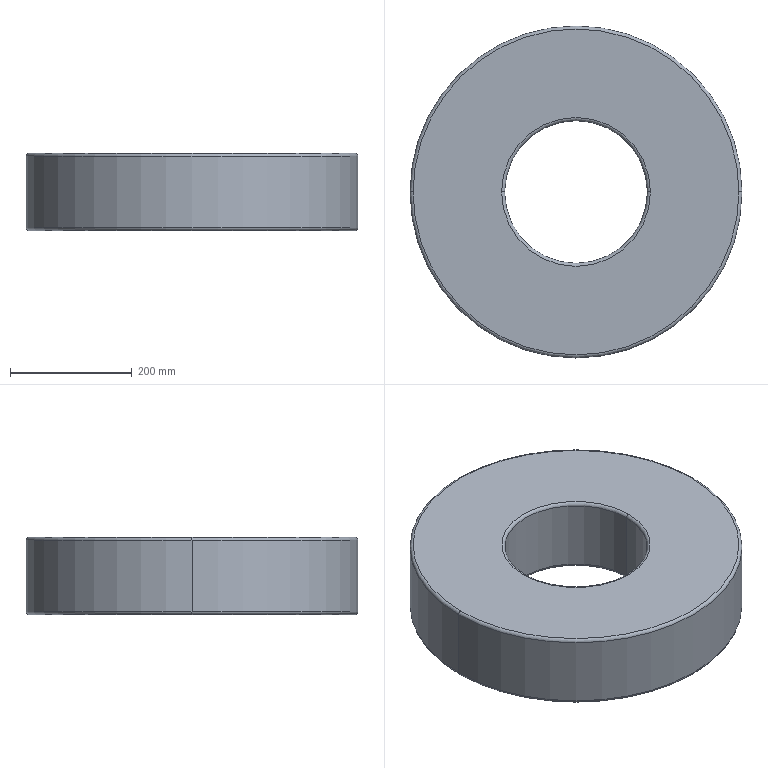Part | SolidWorks | features Extrusion 1, Fillet 1 | 1 solid | 14 faces | box 546.1 x 546.1 x 127 mm | volume 24214209 mm3 | torus 8 | cylinder 4 | plane 2 | commonest cylinder face diameters 234.95 x2 546.1 x2
STEP:
#1=CARTESIAN_POINT('',(-273.05,0.,122.));
#2=VERTEX_POINT('',#1);
#3=CARTESIAN_POINT('',(273.05,0.,122.));
#4=VERTEX_POINT('',#3);
#5=CARTESIAN_POINT('',(0.,0.,122.));
#6=DIRECTION('',(0.,0.,-1.));
#7=DIRECTION('',(1.,0.,0.));
#8=AXIS2_PLACEMENT_3D('',#5,#6,#7);
#9=CIRCLE('',#8,273.05);
#10=EDGE_CURVE('',#2,#4,#9,.T.);
#11=ORIENTED_EDGE('',*,*,#10,.F.);
#12=CARTESIAN_POINT('',(-268.05,0.,127.));
#13=VERTEX_POINT('',#12);
#14=CARTESIAN_POINT('',(-268.05,0.,122.));
#15=DIRECTION('',(0.,1.,0.));
#16=DIRECTION('',(-1.,0.,0.));
#17=AXIS2_PLACEMENT_3D('',#14,#15,#16);
#18=CIRCLE('',#17,5.);
#19=EDGE_CURVE('',#2,#13,#18,.T.);
#20=ORIENTED_EDGE('',*,*,#19,.T.);
#21=CARTESIAN_POINT('',(268.05,0.,127.));
#22=VERTEX_POINT('',#21);
#23=CARTESIAN_POINT('',(0.,0.,127.));
#24=DIRECTION('',(0.,0.,1.));
#25=DIRECTION('',(1.,0.,0.));
#26=AXIS2_PLACEMENT_3D('',#23,#24,#25);
#27=CIRCLE('',#26,268.05);
#28=EDGE_CURVE('',#22,#13,#27,.T.);
#29=ORIENTED_EDGE('',*,*,#28,.F.);
#30=CARTESIAN_POINT('',(268.05,0.,122.));
#31=DIRECTION('',(0.,-1.,0.));
#32=DIRECTION('',(0.,0.,-1.));
#33=AXIS2_PLACEMENT_3D('',#30,#31,#32);
#34=CIRCLE('',#33,5.);
#35=EDGE_CURVE('',#4,#22,#34,.T.);
#36=ORIENTED_EDGE('',*,*,#35,.F.);
#37=EDGE_LOOP('',(#11,#20,#29,#36));
#38=FACE_OUTER_BOUND('',#37,.T.);
#39=CARTESIAN_POINT('',(0.,0.,122.));
#40=DIRECTION('',(0.,0.,1.));
#41=DIRECTION('',(1.,0.,0.));
#42=AXIS2_PLACEMENT_3D('',#39,#40,#41);
#43=TOROIDAL_SURFACE('',#42,268.05,5.);
#44=ADVANCED_FACE('',(#38),#43,.T.);
#45=CARTESIAN_POINT('',(-122.475,0.,127.));
#46=VERTEX_POINT('',#45);
#47=CARTESIAN_POINT('',(122.475,0.,127.));
#48=VERTEX_POINT('',#47);
#49=CARTESIAN_POINT('',(0.,0.,127.));
#50=DIRECTION('',(0.,0.,-1.));
#51=DIRECTION('',(1.,0.,0.));
#52=AXIS2_PLACEMENT_3D('',#49,#50,#51);
#53=CIRCLE('',#52,122.475);
#54=EDGE_CURVE('',#46,#48,#53,.T.);
#55=ORIENTED_EDGE('',*,*,#54,.F.);
#56=CARTESIAN_POINT('',(-117.475,0.,122.));
#57=VERTEX_POINT('',#56);
#58=CARTESIAN_POINT('',(-122.475,0.,122.));
#59=DIRECTION('',(0.,1.,0.));
#60=DIRECTION('',(-1.,0.,0.));
#61=AXIS2_PLACEMENT_3D('',#58,#59,#60);
#62=CIRCLE('',#61,5.);
#63=EDGE_CURVE('',#46,#57,#62,.T.);
#64=ORIENTED_EDGE('',*,*,#63,.T.);
#65=CARTESIAN_POINT('',(117.475,0.,122.));
#66=VERTEX_POINT('',#65);
#67=CARTESIAN_POINT('',(0.,0.,122.));
#68=DIRECTION('',(0.,0.,1.));
#69=DIRECTION('',(1.,0.,0.));
#70=AXIS2_PLACEMENT_3D('',#67,#68,#69);
#71=CIRCLE('',#70,117.475);
#72=EDGE_CURVE('',#66,#57,#71,.T.);
#73=ORIENTED_EDGE('',*,*,#72,.F.);
#74=CARTESIAN_POINT('',(122.475,0.,122.));
#75=DIRECTION('',(0.,-1.,0.));
#76=DIRECTION('',(0.,0.,-1.));
#77=AXIS2_PLACEMENT_3D('',#74,#75,#76);
#78=CIRCLE('',#77,5.);
#79=EDGE_CURVE('',#48,#66,#78,.T.);
#80=ORIENTED_EDGE('',*,*,#79,.F.);
#81=EDGE_LOOP('',(#55,#64,#73,#80));
#82=FACE_OUTER_BOUND('',#81,.T.);
#83=CARTESIAN_POINT('',(0.,0.,122.));
#84=DIRECTION('',(0.,0.,1.));
#85=DIRECTION('',(1.,0.,0.));
#86=AXIS2_PLACEMENT_3D('',#83,#84,#85);
#87=TOROIDAL_SURFACE('',#86,122.475,5.);
#88=ADVANCED_FACE('',(#82),#87,.T.);
#89=CARTESIAN_POINT('',(-117.475,0.,5.));
#90=VERTEX_POINT('',#89);
#91=CARTESIAN_POINT('',(117.475,0.,5.));
#92=VERTEX_POINT('',#91);
#93=CARTESIAN_POINT('',(0.,0.,5.));
#94=DIRECTION('',(0.,0.,-1.));
#95=DIRECTION('',(1.,0.,0.));
#96=AXIS2_PLACEMENT_3D('',#93,#94,#95);
#97=CIRCLE('',#96,117.475);
#98=EDGE_CURVE('',#90,#92,#97,.T.);
#99=ORIENTED_EDGE('',*,*,#98,.F.);
#100=CARTESIAN_POINT('',(-122.475,0.,0.));
#101=VERTEX_POINT('',#100);
#102=CARTESIAN_POINT('',(-122.475,0.,5.));
#103=DIRECTION('',(0.,1.,0.));
#104=DIRECTION('',(-1.,0.,0.));
#105=AXIS2_PLACEMENT_3D('',#102,#103,#104);
#106=CIRCLE('',#105,5.);
#107=EDGE_CURVE('',#90,#101,#106,.T.);
#108=ORIENTED_EDGE('',*,*,#107,.T.);
#109=CARTESIAN_POINT('',(122.475,0.,0.));
#110=VERTEX_POINT('',#109);
#111=CARTESIAN_POINT('',(0.,0.,0.));
#112=DIRECTION('',(0.,0.,1.));
#113=DIRECTION('',(1.,0.,0.));
#114=AXIS2_PLACEMENT_3D('',#111,#112,#113);
#115=CIRCLE('',#114,122.475);
#116=EDGE_CURVE('',#110,#101,#115,.T.);
#117=ORIENTED_EDGE('',*,*,#116,.F.);
#118=CARTESIAN_POINT('',(122.475,0.,5.));
#119=DIRECTION('',(0.,-1.,0.));
#120=DIRECTION('',(0.,0.,-1.));
#121=AXIS2_PLACEMENT_3D('',#118,#119,#120);
#122=CIRCLE('',#121,5.);
#123=EDGE_CURVE('',#92,#110,#122,.T.);
#124=ORIENTED_EDGE('',*,*,#123,.F.);
#125=EDGE_LOOP('',(#99,#108,#117,#124));
#126=FACE_OUTER_BOUND('',#125,.T.);
#127=CARTESIAN_POINT('',(0.,0.,5.));
#128=DIRECTION('',(0.,0.,1.));
#129=DIRECTION('',(1.,0.,0.));
#130=AXIS2_PLACEMENT_3D('',#127,#128,#129);
#131=TOROIDAL_SURFACE('',#130,122.475,5.);
#132=ADVANCED_FACE('',(#126),#131,.T.);
#133=CARTESIAN_POINT('',(-268.05,0.,0.));
#134=VERTEX_POINT('',#133);
#135=CARTESIAN_POINT('',(268.05,0.,0.));
#136=VERTEX_POINT('',#135);
#137=CARTESIAN_POINT('',(0.,0.,0.));
#138=DIRECTION('',(0.,0.,-1.));
#139=DIRECTION('',(1.,0.,0.));
#140=AXIS2_PLACEMENT_3D('',#137,#138,#139);
#141=CIRCLE('',#140,268.05);
#142=EDGE_CURVE('',#134,#136,#141,.T.);
#143=ORIENTED_EDGE('',*,*,#142,.F.);
#144=CARTESIAN_POINT('',(-273.05,0.,5.));
#145=VERTEX_POINT('',#144);
#146=CARTESIAN_POINT('',(-268.05,0.,5.));
#147=DIRECTION('',(0.,1.,0.));
#148=DIRECTION('',(-1.,0.,0.));
#149=AXIS2_PLACEMENT_3D('',#146,#147,#148);
#150=CIRCLE('',#149,5.);
#151=EDGE_CURVE('',#134,#145,#150,.T.);
#152=ORIENTED_EDGE('',*,*,#151,.T.);
#153=CARTESIAN_POINT('',(273.05,0.,5.));
#154=VERTEX_POINT('',#153);
#155=CARTESIAN_POINT('',(0.,0.,5.));
#156=DIRECTION('',(0.,0.,1.));
#157=DIRECTION('',(1.,0.,0.));
#158=AXIS2_PLACEMENT_3D('',#155,#156,#157);
#159=CIRCLE('',#158,273.05);
#160=EDGE_CURVE('',#154,#145,#159,.T.);
#161=ORIENTED_EDGE('',*,*,#160,.F.);
#162=CARTESIAN_POINT('',(268.05,0.,5.));
#163=DIRECTION('',(0.,-1.,0.));
#164=DIRECTION('',(0.,0.,-1.));
#165=AXIS2_PLACEMENT_3D('',#162,#163,#164);
#166=CIRCLE('',#165,5.);
#167=EDGE_CURVE('',#136,#154,#166,.T.);
#168=ORIENTED_EDGE('',*,*,#167,.F.);
#169=EDGE_LOOP('',(#143,#152,#161,#168));
#170=FACE_OUTER_BOUND('',#169,.T.);
#171=CARTESIAN_POINT('',(0.,0.,5.));
#172=DIRECTION('',(0.,0.,1.));
#173=DIRECTION('',(1.,0.,0.));
#174=AXIS2_PLACEMENT_3D('',#171,#172,#173);
#175=TOROIDAL_SURFACE('',#174,268.05,5.);
#176=ADVANCED_FACE('',(#170),#175,.T.);
#177=CARTESIAN_POINT('',(0.,0.,122.));
#178=DIRECTION('',(0.,0.,1.));
#179=DIRECTION('',(1.,0.,0.));
#180=AXIS2_PLACEMENT_3D('',#177,#178,#179);
#181=CIRCLE('',#180,117.475);
#182=EDGE_CURVE('',#57,#66,#181,.T.);
#183=ORIENTED_EDGE('',*,*,#182,.T.);
#184=CARTESIAN_POINT('',(117.475,0.,127.));
#185=DIRECTION('',(0.,0.,-1.));
#186=VECTOR('',#185,1000.);
#187=LINE('',#184,#186);
#188=EDGE_CURVE('',#66,#92,#187,.T.);
#189=ORIENTED_EDGE('',*,*,#188,.T.);
#190=CARTESIAN_POINT('',(0.,0.,5.));
#191=DIRECTION('',(0.,0.,-1.));
#192=DIRECTION('',(1.,0.,0.));
#193=AXIS2_PLACEMENT_3D('',#190,#191,#192);
#194=CIRCLE('',#193,117.475);
#195=EDGE_CURVE('',#92,#90,#194,.T.);
#196=ORIENTED_EDGE('',*,*,#195,.T.);
#197=CARTESIAN_POINT('',(-117.475,0.,127.));
#198=DIRECTION('',(0.,0.,-1.));
#199=VECTOR('',#198,1000.);
#200=LINE('',#197,#199);
#201=EDGE_CURVE('',#57,#90,#200,.T.);
#202=ORIENTED_EDGE('',*,*,#201,.F.);
#203=EDGE_LOOP('',(#183,#189,#196,#202));
#204=FACE_OUTER_BOUND('',#203,.T.);
#205=CARTESIAN_POINT('',(0.,0.,127.));
#206=DIRECTION('',(0.,0.,-1.));
#207=DIRECTION('',(-1.,0.,0.));
#208=AXIS2_PLACEMENT_3D('',#205,#206,#207);
#209=CYLINDRICAL_SURFACE('',#208,117.475);
#210=ADVANCED_FACE('',(#204),#209,.F.);
#211=ORIENTED_EDGE('',*,*,#10,.T.);
#212=CARTESIAN_POINT('',(273.05,0.,127.));
#213=DIRECTION('',(0.,0.,-1.));
#214=VECTOR('',#213,1000.);
#215=LINE('',#212,#214);
#216=EDGE_CURVE('',#4,#154,#215,.T.);
#217=ORIENTED_EDGE('',*,*,#216,.T.);
#218=ORIENTED_EDGE('',*,*,#160,.T.);
#219=CARTESIAN_POINT('',(-273.05,0.,127.));
#220=DIRECTION('',(0.,0.,-1.));
#221=VECTOR('',#220,1000.);
#222=LINE('',#219,#221);
#223=EDGE_CURVE('',#2,#145,#222,.T.);
#224=ORIENTED_EDGE('',*,*,#223,.F.);
#225=EDGE_LOOP('',(#211,#217,#218,#224));
#226=FACE_OUTER_BOUND('',#225,.T.);
#227=CARTESIAN_POINT('',(0.,0.,127.));
#228=DIRECTION('',(0.,0.,-1.));
#229=DIRECTION('',(-1.,0.,0.));
#230=AXIS2_PLACEMENT_3D('',#227,#228,#229);
#231=CYLINDRICAL_SURFACE('',#230,273.05);
#232=ADVANCED_FACE('',(#226),#231,.T.);
#233=CARTESIAN_POINT('',(0.,0.,127.));
#234=DIRECTION('',(0.,0.,-1.));
#235=DIRECTION('',(1.,0.,0.));
#236=AXIS2_PLACEMENT_3D('',#233,#234,#235);
#237=CIRCLE('',#236,122.475);
#238=EDGE_CURVE('',#48,#46,#237,.T.);
#239=ORIENTED_EDGE('',*,*,#238,.T.);
#240=ORIENTED_EDGE('',*,*,#54,.T.);
#241=EDGE_LOOP('',(#239,#240));
#242=FACE_BOUND('',#241,.T.);
#243=ORIENTED_EDGE('',*,*,#28,.T.);
#244=CARTESIAN_POINT('',(0.,0.,127.));
#245=DIRECTION('',(0.,0.,1.));
#246=DIRECTION('',(1.,0.,0.));
#247=AXIS2_PLACEMENT_3D('',#244,#245,#246);
#248=CIRCLE('',#247,268.05);
#249=EDGE_CURVE('',#13,#22,#248,.T.);
#250=ORIENTED_EDGE('',*,*,#249,.T.);
#251=EDGE_LOOP('',(#243,#250));
#252=FACE_OUTER_BOUND('',#251,.T.);
#253=CARTESIAN_POINT('',(0.,0.,127.));
#254=DIRECTION('',(0.,0.,1.));
#255=DIRECTION('',(1.,0.,0.));
#256=AXIS2_PLACEMENT_3D('',#253,#254,#255);
#257=PLANE('',#256);
#258=ADVANCED_FACE('',(#242,#252),#257,.T.);
#259=CARTESIAN_POINT('',(0.,0.,0.));
#260=DIRECTION('',(0.,0.,-1.));
#261=DIRECTION('',(1.,0.,0.));
#262=AXIS2_PLACEMENT_3D('',#259,#260,#261);
#263=CIRCLE('',#262,268.05);
#264=EDGE_CURVE('',#136,#134,#263,.T.);
#265=ORIENTED_EDGE('',*,*,#264,.T.);
#266=ORIENTED_EDGE('',*,*,#142,.T.);
#267=EDGE_LOOP('',(#265,#266));
#268=FACE_OUTER_BOUND('',#267,.T.);
#269=ORIENTED_EDGE('',*,*,#116,.T.);
#270=CARTESIAN_POINT('',(0.,0.,0.));
#271=DIRECTION('',(0.,0.,1.));
#272=DIRECTION('',(1.,0.,0.));
#273=AXIS2_PLACEMENT_3D('',#270,#271,#272);
#274=CIRCLE('',#273,122.475);
#275=EDGE_CURVE('',#101,#110,#274,.T.);
#276=ORIENTED_EDGE('',*,*,#275,.T.);
#277=EDGE_LOOP('',(#269,#276));
#278=FACE_BOUND('',#277,.T.);
#279=CARTESIAN_POINT('',(0.,0.,0.));
#280=DIRECTION('',(0.,0.,1.));
#281=DIRECTION('',(1.,0.,0.));
#282=AXIS2_PLACEMENT_3D('',#279,#280,#281);
#283=PLANE('',#282);
#284=ADVANCED_FACE('',(#268,#278),#283,.F.);
#285=ORIENTED_EDGE('',*,*,#216,.F.);
#286=CARTESIAN_POINT('',(0.,0.,122.));
#287=DIRECTION('',(0.,0.,-1.));
#288=DIRECTION('',(1.,0.,0.));
#289=AXIS2_PLACEMENT_3D('',#286,#287,#288);
#290=CIRCLE('',#289,273.05);
#291=EDGE_CURVE('',#4,#2,#290,.T.);
#292=ORIENTED_EDGE('',*,*,#291,.T.);
#293=ORIENTED_EDGE('',*,*,#223,.T.);
#294=CARTESIAN_POINT('',(0.,0.,5.));
#295=DIRECTION('',(0.,0.,1.));
#296=DIRECTION('',(1.,0.,0.));
#297=AXIS2_PLACEMENT_3D('',#294,#295,#296);
#298=CIRCLE('',#297,273.05);
#299=EDGE_CURVE('',#145,#154,#298,.T.);
#300=ORIENTED_EDGE('',*,*,#299,.T.);
#301=EDGE_LOOP('',(#285,#292,#293,#300));
#302=FACE_OUTER_BOUND('',#301,.T.);
#303=CARTESIAN_POINT('',(0.,0.,127.));
#304=DIRECTION('',(0.,0.,-1.));
#305=DIRECTION('',(-1.,0.,0.));
#306=AXIS2_PLACEMENT_3D('',#303,#304,#305);
#307=CYLINDRICAL_SURFACE('',#306,273.05);
#308=ADVANCED_FACE('',(#302),#307,.T.);
#309=ORIENTED_EDGE('',*,*,#188,.F.);
#310=ORIENTED_EDGE('',*,*,#72,.T.);
#311=ORIENTED_EDGE('',*,*,#201,.T.);
#312=ORIENTED_EDGE('',*,*,#98,.T.);
#313=EDGE_LOOP('',(#309,#310,#311,#312));
#314=FACE_OUTER_BOUND('',#313,.T.);
#315=CARTESIAN_POINT('',(0.,0.,127.));
#316=DIRECTION('',(0.,0.,-1.));
#317=DIRECTION('',(-1.,0.,0.));
#318=AXIS2_PLACEMENT_3D('',#315,#316,#317);
#319=CYLINDRICAL_SURFACE('',#318,117.475);
#320=ADVANCED_FACE('',(#314),#319,.F.);
#321=ORIENTED_EDGE('',*,*,#151,.F.);
#322=ORIENTED_EDGE('',*,*,#264,.F.);
#323=ORIENTED_EDGE('',*,*,#167,.T.);
#324=ORIENTED_EDGE('',*,*,#299,.F.);
#325=EDGE_LOOP('',(#321,#322,#323,#324));
#326=FACE_OUTER_BOUND('',#325,.T.);
#327=CARTESIAN_POINT('',(0.,0.,5.));
#328=DIRECTION('',(0.,0.,1.));
#329=DIRECTION('',(1.,0.,0.));
#330=AXIS2_PLACEMENT_3D('',#327,#328,#329);
#331=TOROIDAL_SURFACE('',#330,268.05,5.);
#332=ADVANCED_FACE('',(#326),#331,.T.);
#333=ORIENTED_EDGE('',*,*,#107,.F.);
#334=ORIENTED_EDGE('',*,*,#195,.F.);
#335=ORIENTED_EDGE('',*,*,#123,.T.);
#336=ORIENTED_EDGE('',*,*,#275,.F.);
#337=EDGE_LOOP('',(#333,#334,#335,#336));
#338=FACE_OUTER_BOUND('',#337,.T.);
#339=CARTESIAN_POINT('',(0.,0.,5.));
#340=DIRECTION('',(0.,0.,1.));
#341=DIRECTION('',(1.,0.,0.));
#342=AXIS2_PLACEMENT_3D('',#339,#340,#341);
#343=TOROIDAL_SURFACE('',#342,122.475,5.);
#344=ADVANCED_FACE('',(#338),#343,.T.);
#345=ORIENTED_EDGE('',*,*,#63,.F.);
#346=ORIENTED_EDGE('',*,*,#238,.F.);
#347=ORIENTED_EDGE('',*,*,#79,.T.);
#348=ORIENTED_EDGE('',*,*,#182,.F.);
#349=EDGE_LOOP('',(#345,#346,#347,#348));
#350=FACE_OUTER_BOUND('',#349,.T.);
#351=CARTESIAN_POINT('',(0.,0.,122.));
#352=DIRECTION('',(0.,0.,1.));
#353=DIRECTION('',(1.,0.,0.));
#354=AXIS2_PLACEMENT_3D('',#351,#352,#353);
#355=TOROIDAL_SURFACE('',#354,122.475,5.);
#356=ADVANCED_FACE('',(#350),#355,.T.);
#357=ORIENTED_EDGE('',*,*,#19,.F.);
#358=ORIENTED_EDGE('',*,*,#291,.F.);
#359=ORIENTED_EDGE('',*,*,#35,.T.);
#360=ORIENTED_EDGE('',*,*,#249,.F.);
#361=EDGE_LOOP('',(#357,#358,#359,#360));
#362=FACE_OUTER_BOUND('',#361,.T.);
#363=CARTESIAN_POINT('',(0.,0.,122.));
#364=DIRECTION('',(0.,0.,1.));
#365=DIRECTION('',(1.,0.,0.));
#366=AXIS2_PLACEMENT_3D('',#363,#364,#365);
#367=TOROIDAL_SURFACE('',#366,268.05,5.);
#368=ADVANCED_FACE('',(#362),#367,.T.);
#369=CLOSED_SHELL('',(#44,#88,#132,#176,#210,#232,#258,#284,#308,#320,#332,#344,#356,#368));
#370=MANIFOLD_SOLID_BREP('',#369);
#371=CARTESIAN_POINT('',(0.,0.,0.));
#372=DIRECTION('',(0.,0.,1.));
#373=DIRECTION('',(1.,0.,0.));
#374=AXIS2_PLACEMENT_3D('',#371,#372,#373);
#375=(LENGTH_UNIT()NAMED_UNIT(*)SI_UNIT(.MILLI.,.METRE.));
#376=UNCERTAINTY_MEASURE_WITH_UNIT(LENGTH_MEASURE(0.00001),#375,'','');
#377=(NAMED_UNIT(*)PLANE_ANGLE_UNIT()SI_UNIT($,.RADIAN.));
#378=(NAMED_UNIT(*)SI_UNIT($,.STERADIAN.)SOLID_ANGLE_UNIT());
#379=(GEOMETRIC_REPRESENTATION_CONTEXT(3)GLOBAL_UNCERTAINTY_ASSIGNED_CONTEXT((#376))GLOBAL_UNIT_ASSIGNED_CONTEXT((#375,#377,#378))REPRESENTATION_CONTEXT('',''));
#380=ADVANCED_BREP_SHAPE_REPRESENTATION('',(#370,#374),#379);